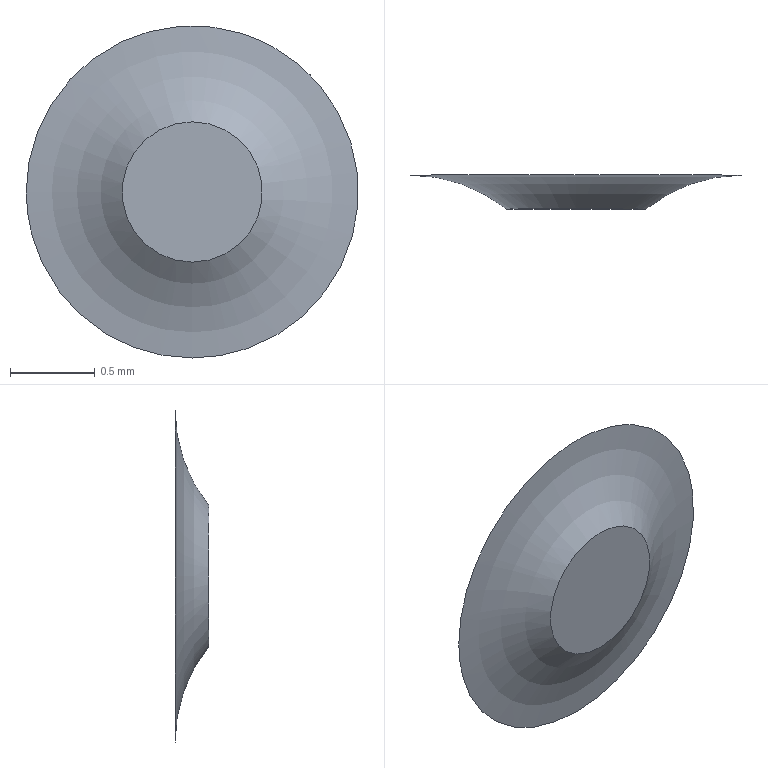Part | STEP file | Basler ace 2 USB3-1-1-1_5 | 1 solid | 3 faces | box 1.96 x 0.2 x 1.96 mm | volume 0.2322 mm3 | plane 2 | torus 1
STEP:
#1=CARTESIAN_POINT('',(10.5,14.2,-24.164));
#2=VERTEX_POINT('',#1);
#3=CARTESIAN_POINT('',(10.5,14.2,-23.75));
#4=DIRECTION('',(0.,1.,0.));
#5=DIRECTION('',(0.,0.,1.));
#6=AXIS2_PLACEMENT_3D('',#3,#4,#5);
#7=CIRCLE('',#6,0.4141);
#8=EDGE_CURVE('',#2,#2,#7,.F.);
#9=ORIENTED_EDGE('',*,*,#8,.T.);
#10=EDGE_LOOP('',(#9));
#11=FACE_OUTER_BOUND('',#10,.T.);
#12=CARTESIAN_POINT('',(-14.2,14.2,0.));
#13=DIRECTION('',(0.,1.,0.));
#14=DIRECTION('',(0.,0.,1.));
#15=AXIS2_PLACEMENT_3D('',#12,#13,#14);
#16=PLANE('',#15);
#17=ADVANCED_FACE('',(#11),#16,.F.);
#18=CARTESIAN_POINT('',(9.52,14.4,-23.75));
#19=VERTEX_POINT('',#18);
#20=CARTESIAN_POINT('',(10.5,14.4,-24.73));
#21=VERTEX_POINT('',#20);
#22=CARTESIAN_POINT('',(9.52,14.4,-23.75));
#23=CARTESIAN_POINT('',(9.52,14.4,-23.686));
#24=CARTESIAN_POINT('',(9.533,14.4,-23.558));
#25=CARTESIAN_POINT('',(9.589,14.4,-23.373));
#26=CARTESIAN_POINT('',(9.68,14.4,-23.202));
#27=CARTESIAN_POINT('',(9.803,14.4,-23.053));
#28=CARTESIAN_POINT('',(9.952,14.4,-22.93));
#29=CARTESIAN_POINT('',(10.123,14.4,-22.839));
#30=CARTESIAN_POINT('',(10.307,14.4,-22.782));
#31=CARTESIAN_POINT('',(10.5,14.4,-22.764));
#32=CARTESIAN_POINT('',(10.692,14.4,-22.782));
#33=CARTESIAN_POINT('',(10.877,14.4,-22.839));
#34=CARTESIAN_POINT('',(11.048,14.4,-22.93));
#35=CARTESIAN_POINT('',(11.197,14.4,-23.053));
#36=CARTESIAN_POINT('',(11.32,14.4,-23.202));
#37=CARTESIAN_POINT('',(11.411,14.4,-23.373));
#38=CARTESIAN_POINT('',(11.468,14.4,-23.557));
#39=CARTESIAN_POINT('',(11.486,14.4,-23.75));
#40=CARTESIAN_POINT('',(11.468,14.4,-23.942));
#41=CARTESIAN_POINT('',(11.411,14.4,-24.127));
#42=CARTESIAN_POINT('',(11.32,14.4,-24.298));
#43=CARTESIAN_POINT('',(11.197,14.4,-24.447));
#44=CARTESIAN_POINT('',(11.048,14.4,-24.57));
#45=CARTESIAN_POINT('',(10.877,14.4,-24.661));
#46=CARTESIAN_POINT('',(10.693,14.4,-24.718));
#47=CARTESIAN_POINT('',(10.564,14.4,-24.73));
#48=CARTESIAN_POINT('',(10.5,14.4,-24.73));
#49=B_SPLINE_CURVE_WITH_KNOTS('',3,(#22,#23,#24,#25,#26,#27,#28,#29,#30,#31,#32,#33,#34,#35,#36,#37,#38,#39,#40,#41,#42,#43,#44,#45,#46,#47,#48),.UNSPECIFIED.,.F.,.F.,(4,1,1,1,1,1,1,1,1,1,1,1,1,1,1,1,1,1,1,1,1,1,1,1,4),(0.,0.03123,0.0625,0.0937,0.125,0.1562,0.1875,0.2187,0.25,0.2812,0.3125,0.3437,0.375,0.4062,0.4375,0.4687,0.5,0.5312,0.5625,0.5937,0.625,0.6562,0.6875,0.7187,0.75),.UNSPECIFIED.);
#50=EDGE_CURVE('',#19,#21,#49,.T.);
#51=ORIENTED_EDGE('',*,*,#50,.F.);
#52=CARTESIAN_POINT('',(10.5,14.4,-24.73));
#53=CARTESIAN_POINT('',(10.436,14.4,-24.73));
#54=CARTESIAN_POINT('',(10.308,14.4,-24.718));
#55=CARTESIAN_POINT('',(10.123,14.4,-24.661));
#56=CARTESIAN_POINT('',(9.952,14.4,-24.57));
#57=CARTESIAN_POINT('',(9.803,14.4,-24.447));
#58=CARTESIAN_POINT('',(9.68,14.4,-24.298));
#59=CARTESIAN_POINT('',(9.589,14.4,-24.127));
#60=CARTESIAN_POINT('',(9.532,14.4,-23.943));
#61=CARTESIAN_POINT('',(9.52,14.4,-23.814));
#62=CARTESIAN_POINT('',(9.52,14.4,-23.75));
#63=B_SPLINE_CURVE_WITH_KNOTS('',3,(#52,#53,#54,#55,#56,#57,#58,#59,#60,#61,#62),.UNSPECIFIED.,.F.,.F.,(4,1,1,1,1,1,1,1,4),(0.75,0.7812,0.8125,0.8437,0.875,0.9062,0.9375,0.9687,1.),.UNSPECIFIED.);
#64=EDGE_CURVE('',#21,#19,#63,.T.);
#65=ORIENTED_EDGE('',*,*,#64,.F.);
#66=CARTESIAN_POINT('',(10.5,13.5,-24.73));
#67=DIRECTION('',(1.,0.,0.));
#68=DIRECTION('',(0.,0.,-1.));
#69=AXIS2_PLACEMENT_3D('',#66,#67,#68);
#70=CIRCLE('',#69,0.9);
#71=EDGE_CURVE('',#21,#2,#70,.T.);
#72=ORIENTED_EDGE('',*,*,#71,.T.);
#73=ORIENTED_EDGE('',*,*,#8,.F.);
#74=ORIENTED_EDGE('',*,*,#71,.F.);
#75=EDGE_LOOP('',(#51,#65,#72,#73,#74));
#76=FACE_OUTER_BOUND('',#75,.T.);
#77=CARTESIAN_POINT('',(10.5,13.5,-23.75));
#78=DIRECTION('',(0.,1.,0.));
#79=DIRECTION('',(0.,0.,1.));
#80=AXIS2_PLACEMENT_3D('',#77,#78,#79);
#81=TOROIDAL_SURFACE('',#80,0.9798,0.9);
#82=ADVANCED_FACE('',(#76),#81,.F.);
#83=ORIENTED_EDGE('',*,*,#50,.T.);
#84=ORIENTED_EDGE('',*,*,#64,.T.);
#85=EDGE_LOOP('',(#83,#84));
#86=FACE_OUTER_BOUND('',#85,.T.);
#87=CARTESIAN_POINT('',(0.,14.4,-14.975));
#88=DIRECTION('',(0.,1.,0.));
#89=DIRECTION('',(0.,0.,1.));
#90=AXIS2_PLACEMENT_3D('',#87,#88,#89);
#91=PLANE('',#90);
#92=ADVANCED_FACE('',(#86),#91,.T.);
#93=CLOSED_SHELL('',(#17,#82,#92));
#94=MANIFOLD_SOLID_BREP('',#93);
#95=(LENGTH_UNIT()NAMED_UNIT(*)SI_UNIT(.MILLI.,.METRE.));
#96=UNCERTAINTY_MEASURE_WITH_UNIT(LENGTH_MEASURE(0.01),#95,'','');
#97=(NAMED_UNIT(*)PLANE_ANGLE_UNIT()SI_UNIT($,.RADIAN.));
#98=(NAMED_UNIT(*)SI_UNIT($,.STERADIAN.)SOLID_ANGLE_UNIT());
#99=(GEOMETRIC_REPRESENTATION_CONTEXT(3)GLOBAL_UNCERTAINTY_ASSIGNED_CONTEXT((#96))GLOBAL_UNIT_ASSIGNED_CONTEXT((#95,#97,#98))REPRESENTATION_CONTEXT('',''));
#100=ADVANCED_BREP_SHAPE_REPRESENTATION('',(#94),#99);